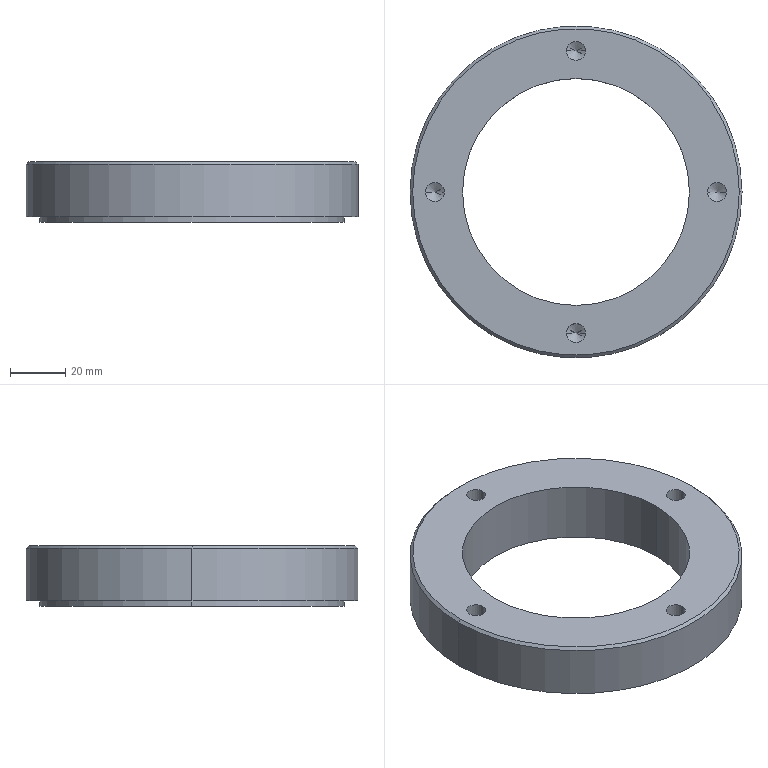Part | SolidWorks | features Chamfer 1, CirPattern 1, FlatPattern 1, HoleWzd 1, ICE 1, SMBaseFlange 1, SheetMetal 1 | 1 solid | 27 faces | box 120 x 120 x 22 mm | volume 125864 mm3 | cylinder 14 | cone 10 | plane 3 | commonest cylinder face diameters 6.8 x8 82 x2 110 x2 120 x2
STEP:
#1=CARTESIAN_POINT('',(-3.4,51.,-19.75));
#2=VERTEX_POINT('',#1);
#3=CARTESIAN_POINT('',(3.4,51.,-19.75));
#4=VERTEX_POINT('',#3);
#5=CARTESIAN_POINT('',(0.,51.,-19.75));
#6=DIRECTION('',(0.,0.,1.));
#7=DIRECTION('',(1.,0.,0.));
#8=AXIS2_PLACEMENT_3D('',#5,#6,#7);
#9=CIRCLE('',#8,3.4);
#10=EDGE_CURVE('',#2,#4,#9,.T.);
#11=ORIENTED_EDGE('',*,*,#10,.F.);
#12=CARTESIAN_POINT('',(-3.4,51.,0.));
#13=VERTEX_POINT('',#12);
#14=CARTESIAN_POINT('',(-3.4,51.,0.));
#15=DIRECTION('',(0.,0.,1.));
#16=VECTOR('',#15,1000.);
#17=LINE('',#14,#16);
#18=EDGE_CURVE('',#2,#13,#17,.T.);
#19=ORIENTED_EDGE('',*,*,#18,.T.);
#20=CARTESIAN_POINT('',(3.4,51.,0.));
#21=VERTEX_POINT('',#20);
#22=CARTESIAN_POINT('',(0.,51.,0.));
#23=DIRECTION('',(0.,0.,1.));
#24=DIRECTION('',(1.,0.,0.));
#25=AXIS2_PLACEMENT_3D('',#22,#23,#24);
#26=CIRCLE('',#25,3.4);
#27=EDGE_CURVE('',#13,#21,#26,.T.);
#28=ORIENTED_EDGE('',*,*,#27,.T.);
#29=CARTESIAN_POINT('',(3.4,51.,0.));
#30=DIRECTION('',(0.,0.,1.));
#31=VECTOR('',#30,1000.);
#32=LINE('',#29,#31);
#33=EDGE_CURVE('',#4,#21,#32,.T.);
#34=ORIENTED_EDGE('',*,*,#33,.F.);
#35=EDGE_LOOP('',(#11,#19,#28,#34));
#36=FACE_OUTER_BOUND('',#35,.T.);
#37=CARTESIAN_POINT('',(0.,51.,0.));
#38=DIRECTION('',(0.,0.,1.));
#39=DIRECTION('',(1.,0.,0.));
#40=AXIS2_PLACEMENT_3D('',#37,#38,#39);
#41=CYLINDRICAL_SURFACE('',#40,3.4);
#42=ADVANCED_FACE('',(#36),#41,.F.);
#43=CARTESIAN_POINT('',(0.,51.,-21.793));
#44=VERTEX_POINT('',#43);
#45=CARTESIAN_POINT('',(3.4,51.,-19.75));
#46=DIRECTION('',(0.8572,0.,0.515));
#47=VECTOR('',#46,1000.);
#48=LINE('',#45,#47);
#49=EDGE_CURVE('',#44,#4,#48,.T.);
#50=ORIENTED_EDGE('',*,*,#49,.F.);
#51=CARTESIAN_POINT('',(-3.4,51.,-19.75));
#52=DIRECTION('',(-0.8572,0.,0.515));
#53=VECTOR('',#52,1000.);
#54=LINE('',#51,#53);
#55=EDGE_CURVE('',#44,#2,#54,.T.);
#56=ORIENTED_EDGE('',*,*,#55,.T.);
#57=ORIENTED_EDGE('',*,*,#10,.T.);
#58=EDGE_LOOP('',(#50,#56,#57));
#59=FACE_OUTER_BOUND('',#58,.T.);
#60=CARTESIAN_POINT('',(0.,51.,-19.75));
#61=DIRECTION('',(0.,0.,1.));
#62=DIRECTION('',(1.,0.,0.));
#63=AXIS2_PLACEMENT_3D('',#60,#61,#62);
#64=CONICAL_SURFACE('',#63,3.4,1.03);
#65=ADVANCED_FACE('',(#59),#64,.F.);
#66=CARTESIAN_POINT('',(-54.4,0.,-19.75));
#67=VERTEX_POINT('',#66);
#68=CARTESIAN_POINT('',(-47.6,0.,-19.75));
#69=VERTEX_POINT('',#68);
#70=CARTESIAN_POINT('',(-51.,0.,-19.75));
#71=DIRECTION('',(0.,0.,1.));
#72=DIRECTION('',(1.,0.,0.));
#73=AXIS2_PLACEMENT_3D('',#70,#71,#72);
#74=CIRCLE('',#73,3.4);
#75=EDGE_CURVE('',#67,#69,#74,.T.);
#76=ORIENTED_EDGE('',*,*,#75,.F.);
#77=CARTESIAN_POINT('',(-54.4,0.,0.));
#78=VERTEX_POINT('',#77);
#79=CARTESIAN_POINT('',(-54.4,0.,0.));
#80=DIRECTION('',(0.,0.,1.));
#81=VECTOR('',#80,1000.);
#82=LINE('',#79,#81);
#83=EDGE_CURVE('',#67,#78,#82,.T.);
#84=ORIENTED_EDGE('',*,*,#83,.T.);
#85=CARTESIAN_POINT('',(-47.6,0.,0.));
#86=VERTEX_POINT('',#85);
#87=CARTESIAN_POINT('',(-51.,0.,0.));
#88=DIRECTION('',(0.,0.,1.));
#89=DIRECTION('',(1.,0.,0.));
#90=AXIS2_PLACEMENT_3D('',#87,#88,#89);
#91=CIRCLE('',#90,3.4);
#92=EDGE_CURVE('',#78,#86,#91,.T.);
#93=ORIENTED_EDGE('',*,*,#92,.T.);
#94=CARTESIAN_POINT('',(-47.6,0.,0.));
#95=DIRECTION('',(0.,0.,1.));
#96=VECTOR('',#95,1000.);
#97=LINE('',#94,#96);
#98=EDGE_CURVE('',#69,#86,#97,.T.);
#99=ORIENTED_EDGE('',*,*,#98,.F.);
#100=EDGE_LOOP('',(#76,#84,#93,#99));
#101=FACE_OUTER_BOUND('',#100,.T.);
#102=CARTESIAN_POINT('',(-51.,0.,0.));
#103=DIRECTION('',(0.,0.,1.));
#104=DIRECTION('',(1.,0.,0.));
#105=AXIS2_PLACEMENT_3D('',#102,#103,#104);
#106=CYLINDRICAL_SURFACE('',#105,3.4);
#107=ADVANCED_FACE('',(#101),#106,.F.);
#108=CARTESIAN_POINT('',(-51.,0.,-21.793));
#109=VERTEX_POINT('',#108);
#110=CARTESIAN_POINT('',(-47.6,0.,-19.75));
#111=DIRECTION('',(0.8572,0.,0.515));
#112=VECTOR('',#111,1000.);
#113=LINE('',#110,#112);
#114=EDGE_CURVE('',#109,#69,#113,.T.);
#115=ORIENTED_EDGE('',*,*,#114,.F.);
#116=CARTESIAN_POINT('',(-54.4,0.,-19.75));
#117=DIRECTION('',(-0.8572,0.,0.515));
#118=VECTOR('',#117,1000.);
#119=LINE('',#116,#118);
#120=EDGE_CURVE('',#109,#67,#119,.T.);
#121=ORIENTED_EDGE('',*,*,#120,.T.);
#122=ORIENTED_EDGE('',*,*,#75,.T.);
#123=EDGE_LOOP('',(#115,#121,#122));
#124=FACE_OUTER_BOUND('',#123,.T.);
#125=CARTESIAN_POINT('',(-51.,0.,-19.75));
#126=DIRECTION('',(0.,0.,1.));
#127=DIRECTION('',(1.,0.,0.));
#128=AXIS2_PLACEMENT_3D('',#125,#126,#127);
#129=CONICAL_SURFACE('',#128,3.4,1.03);
#130=ADVANCED_FACE('',(#124),#129,.F.);
#131=CARTESIAN_POINT('',(-3.4,-51.,-19.75));
#132=VERTEX_POINT('',#131);
#133=CARTESIAN_POINT('',(3.4,-51.,-19.75));
#134=VERTEX_POINT('',#133);
#135=CARTESIAN_POINT('',(0.,-51.,-19.75));
#136=DIRECTION('',(0.,0.,1.));
#137=DIRECTION('',(1.,0.,0.));
#138=AXIS2_PLACEMENT_3D('',#135,#136,#137);
#139=CIRCLE('',#138,3.4);
#140=EDGE_CURVE('',#132,#134,#139,.T.);
#141=ORIENTED_EDGE('',*,*,#140,.F.);
#142=CARTESIAN_POINT('',(-3.4,-51.,0.));
#143=VERTEX_POINT('',#142);
#144=CARTESIAN_POINT('',(-3.4,-51.,0.));
#145=DIRECTION('',(0.,0.,1.));
#146=VECTOR('',#145,1000.);
#147=LINE('',#144,#146);
#148=EDGE_CURVE('',#132,#143,#147,.T.);
#149=ORIENTED_EDGE('',*,*,#148,.T.);
#150=CARTESIAN_POINT('',(3.4,-51.,0.));
#151=VERTEX_POINT('',#150);
#152=CARTESIAN_POINT('',(0.,-51.,0.));
#153=DIRECTION('',(0.,0.,1.));
#154=DIRECTION('',(1.,0.,0.));
#155=AXIS2_PLACEMENT_3D('',#152,#153,#154);
#156=CIRCLE('',#155,3.4);
#157=EDGE_CURVE('',#143,#151,#156,.T.);
#158=ORIENTED_EDGE('',*,*,#157,.T.);
#159=CARTESIAN_POINT('',(3.4,-51.,0.));
#160=DIRECTION('',(0.,0.,1.));
#161=VECTOR('',#160,1000.);
#162=LINE('',#159,#161);
#163=EDGE_CURVE('',#134,#151,#162,.T.);
#164=ORIENTED_EDGE('',*,*,#163,.F.);
#165=EDGE_LOOP('',(#141,#149,#158,#164));
#166=FACE_OUTER_BOUND('',#165,.T.);
#167=CARTESIAN_POINT('',(0.,-51.,0.));
#168=DIRECTION('',(0.,0.,1.));
#169=DIRECTION('',(1.,0.,0.));
#170=AXIS2_PLACEMENT_3D('',#167,#168,#169);
#171=CYLINDRICAL_SURFACE('',#170,3.4);
#172=ADVANCED_FACE('',(#166),#171,.F.);
#173=CARTESIAN_POINT('',(0.,-51.,-21.793));
#174=VERTEX_POINT('',#173);
#175=CARTESIAN_POINT('',(3.4,-51.,-19.75));
#176=DIRECTION('',(0.8572,0.,0.515));
#177=VECTOR('',#176,1000.);
#178=LINE('',#175,#177);
#179=EDGE_CURVE('',#174,#134,#178,.T.);
#180=ORIENTED_EDGE('',*,*,#179,.F.);
#181=CARTESIAN_POINT('',(-3.4,-51.,-19.75));
#182=DIRECTION('',(-0.8572,0.,0.515));
#183=VECTOR('',#182,1000.);
#184=LINE('',#181,#183);
#185=EDGE_CURVE('',#174,#132,#184,.T.);
#186=ORIENTED_EDGE('',*,*,#185,.T.);
#187=ORIENTED_EDGE('',*,*,#140,.T.);
#188=EDGE_LOOP('',(#180,#186,#187));
#189=FACE_OUTER_BOUND('',#188,.T.);
#190=CARTESIAN_POINT('',(0.,-51.,-19.75));
#191=DIRECTION('',(0.,0.,1.));
#192=DIRECTION('',(1.,0.,0.));
#193=AXIS2_PLACEMENT_3D('',#190,#191,#192);
#194=CONICAL_SURFACE('',#193,3.4,1.03);
#195=ADVANCED_FACE('',(#189),#194,.F.);
#196=CARTESIAN_POINT('',(47.6,0.,-19.75));
#197=VERTEX_POINT('',#196);
#198=CARTESIAN_POINT('',(54.4,0.,-19.75));
#199=VERTEX_POINT('',#198);
#200=CARTESIAN_POINT('',(51.,0.,-19.75));
#201=DIRECTION('',(0.,0.,1.));
#202=DIRECTION('',(1.,0.,0.));
#203=AXIS2_PLACEMENT_3D('',#200,#201,#202);
#204=CIRCLE('',#203,3.4);
#205=EDGE_CURVE('',#197,#199,#204,.T.);
#206=ORIENTED_EDGE('',*,*,#205,.F.);
#207=CARTESIAN_POINT('',(47.6,0.,0.));
#208=VERTEX_POINT('',#207);
#209=CARTESIAN_POINT('',(47.6,0.,0.));
#210=DIRECTION('',(0.,0.,1.));
#211=VECTOR('',#210,1000.);
#212=LINE('',#209,#211);
#213=EDGE_CURVE('',#197,#208,#212,.T.);
#214=ORIENTED_EDGE('',*,*,#213,.T.);
#215=CARTESIAN_POINT('',(54.4,0.,0.));
#216=VERTEX_POINT('',#215);
#217=CARTESIAN_POINT('',(51.,0.,0.));
#218=DIRECTION('',(0.,0.,1.));
#219=DIRECTION('',(1.,0.,0.));
#220=AXIS2_PLACEMENT_3D('',#217,#218,#219);
#221=CIRCLE('',#220,3.4);
#222=EDGE_CURVE('',#208,#216,#221,.T.);
#223=ORIENTED_EDGE('',*,*,#222,.T.);
#224=CARTESIAN_POINT('',(54.4,0.,0.));
#225=DIRECTION('',(0.,0.,1.));
#226=VECTOR('',#225,1000.);
#227=LINE('',#224,#226);
#228=EDGE_CURVE('',#199,#216,#227,.T.);
#229=ORIENTED_EDGE('',*,*,#228,.F.);
#230=EDGE_LOOP('',(#206,#214,#223,#229));
#231=FACE_OUTER_BOUND('',#230,.T.);
#232=CARTESIAN_POINT('',(51.,0.,0.));
#233=DIRECTION('',(0.,0.,1.));
#234=DIRECTION('',(1.,0.,0.));
#235=AXIS2_PLACEMENT_3D('',#232,#233,#234);
#236=CYLINDRICAL_SURFACE('',#235,3.4);
#237=ADVANCED_FACE('',(#231),#236,.F.);
#238=CARTESIAN_POINT('',(51.,0.,-21.793));
#239=VERTEX_POINT('',#238);
#240=CARTESIAN_POINT('',(54.4,0.,-19.75));
#241=DIRECTION('',(0.8572,0.,0.515));
#242=VECTOR('',#241,1000.);
#243=LINE('',#240,#242);
#244=EDGE_CURVE('',#239,#199,#243,.T.);
#245=ORIENTED_EDGE('',*,*,#244,.F.);
#246=CARTESIAN_POINT('',(47.6,0.,-19.75));
#247=DIRECTION('',(-0.8572,0.,0.515));
#248=VECTOR('',#247,1000.);
#249=LINE('',#246,#248);
#250=EDGE_CURVE('',#239,#197,#249,.T.);
#251=ORIENTED_EDGE('',*,*,#250,.T.);
#252=ORIENTED_EDGE('',*,*,#205,.T.);
#253=EDGE_LOOP('',(#245,#251,#252));
#254=FACE_OUTER_BOUND('',#253,.T.);
#255=CARTESIAN_POINT('',(51.,0.,-19.75));
#256=DIRECTION('',(0.,0.,1.));
#257=DIRECTION('',(1.,0.,0.));
#258=AXIS2_PLACEMENT_3D('',#255,#256,#257);
#259=CONICAL_SURFACE('',#258,3.4,1.03);
#260=ADVANCED_FACE('',(#254),#259,.F.);
#261=CARTESIAN_POINT('',(59.,0.,0.));
#262=VERTEX_POINT('',#261);
#263=CARTESIAN_POINT('',(-59.,0.,0.));
#264=VERTEX_POINT('',#263);
#265=CARTESIAN_POINT('',(0.,0.,0.));
#266=DIRECTION('',(0.,0.,1.));
#267=DIRECTION('',(1.,0.,0.));
#268=AXIS2_PLACEMENT_3D('',#265,#266,#267);
#269=CIRCLE('',#268,59.);
#270=EDGE_CURVE('',#262,#264,#269,.T.);
#271=ORIENTED_EDGE('',*,*,#270,.F.);
#272=CARTESIAN_POINT('',(60.,0.,-1.));
#273=VERTEX_POINT('',#272);
#274=CARTESIAN_POINT('',(59.,0.,0.));
#275=DIRECTION('',(0.7071,0.,-0.7071));
#276=VECTOR('',#275,1000.);
#277=LINE('',#274,#276);
#278=EDGE_CURVE('',#262,#273,#277,.T.);
#279=ORIENTED_EDGE('',*,*,#278,.T.);
#280=CARTESIAN_POINT('',(-60.,0.,-1.));
#281=VERTEX_POINT('',#280);
#282=CARTESIAN_POINT('',(0.,0.,-1.));
#283=DIRECTION('',(0.,0.,-1.));
#284=DIRECTION('',(1.,0.,0.));
#285=AXIS2_PLACEMENT_3D('',#282,#283,#284);
#286=CIRCLE('',#285,60.);
#287=EDGE_CURVE('',#281,#273,#286,.T.);
#288=ORIENTED_EDGE('',*,*,#287,.F.);
#289=CARTESIAN_POINT('',(-59.,0.,0.));
#290=DIRECTION('',(-0.7071,0.,-0.7071));
#291=VECTOR('',#290,1000.);
#292=LINE('',#289,#291);
#293=EDGE_CURVE('',#264,#281,#292,.T.);
#294=ORIENTED_EDGE('',*,*,#293,.F.);
#295=EDGE_LOOP('',(#271,#279,#288,#294));
#296=FACE_OUTER_BOUND('',#295,.T.);
#297=CARTESIAN_POINT('',(0.,0.,0.));
#298=DIRECTION('',(0.,0.,-1.));
#299=DIRECTION('',(-1.,0.,0.));
#300=AXIS2_PLACEMENT_3D('',#297,#298,#299);
#301=CONICAL_SURFACE('',#300,59.,0.7854);
#302=ADVANCED_FACE('',(#296),#301,.T.);
#303=CARTESIAN_POINT('',(-55.,0.,-22.));
#304=VERTEX_POINT('',#303);
#305=CARTESIAN_POINT('',(55.,0.,-22.));
#306=VERTEX_POINT('',#305);
#307=CARTESIAN_POINT('',(0.,0.,-22.));
#308=DIRECTION('',(0.,0.,-1.));
#309=DIRECTION('',(-1.,0.,0.));
#310=AXIS2_PLACEMENT_3D('',#307,#308,#309);
#311=CIRCLE('',#310,55.);
#312=EDGE_CURVE('',#304,#306,#311,.T.);
#313=ORIENTED_EDGE('',*,*,#312,.F.);
#314=CARTESIAN_POINT('',(-55.,0.,-20.));
#315=VERTEX_POINT('',#314);
#316=CARTESIAN_POINT('',(-55.,0.,-22.));
#317=DIRECTION('',(0.,0.,1.));
#318=VECTOR('',#317,1000.);
#319=LINE('',#316,#318);
#320=EDGE_CURVE('',#304,#315,#319,.T.);
#321=ORIENTED_EDGE('',*,*,#320,.T.);
#322=CARTESIAN_POINT('',(55.,0.,-20.));
#323=VERTEX_POINT('',#322);
#324=CARTESIAN_POINT('',(0.,0.,-20.));
#325=DIRECTION('',(0.,0.,-1.));
#326=DIRECTION('',(-1.,0.,0.));
#327=AXIS2_PLACEMENT_3D('',#324,#325,#326);
#328=CIRCLE('',#327,55.);
#329=EDGE_CURVE('',#315,#323,#328,.T.);
#330=ORIENTED_EDGE('',*,*,#329,.T.);
#331=CARTESIAN_POINT('',(55.,0.,-22.));
#332=DIRECTION('',(0.,0.,1.));
#333=VECTOR('',#332,1000.);
#334=LINE('',#331,#333);
#335=EDGE_CURVE('',#306,#323,#334,.T.);
#336=ORIENTED_EDGE('',*,*,#335,.F.);
#337=EDGE_LOOP('',(#313,#321,#330,#336));
#338=FACE_OUTER_BOUND('',#337,.T.);
#339=CARTESIAN_POINT('',(0.,0.,-22.));
#340=DIRECTION('',(0.,0.,1.));
#341=DIRECTION('',(1.,0.,0.));
#342=AXIS2_PLACEMENT_3D('',#339,#340,#341);
#343=CYLINDRICAL_SURFACE('',#342,55.);
#344=ADVANCED_FACE('',(#338),#343,.T.);
#345=CARTESIAN_POINT('',(41.,0.,-22.));
#346=VERTEX_POINT('',#345);
#347=CARTESIAN_POINT('',(-41.,0.,-22.));
#348=VERTEX_POINT('',#347);
#349=CARTESIAN_POINT('',(0.,0.,-22.));
#350=DIRECTION('',(0.,0.,-1.));
#351=DIRECTION('',(-1.,0.,0.));
#352=AXIS2_PLACEMENT_3D('',#349,#350,#351);
#353=CIRCLE('',#352,41.);
#354=EDGE_CURVE('',#346,#348,#353,.T.);
#355=ORIENTED_EDGE('',*,*,#354,.T.);
#356=CARTESIAN_POINT('',(-41.,0.,0.));
#357=VERTEX_POINT('',#356);
#358=CARTESIAN_POINT('',(-41.,0.,-20.));
#359=DIRECTION('',(0.,0.,1.));
#360=VECTOR('',#359,1000.);
#361=LINE('',#358,#360);
#362=EDGE_CURVE('',#348,#357,#361,.T.);
#363=ORIENTED_EDGE('',*,*,#362,.T.);
#364=CARTESIAN_POINT('',(41.,0.,0.));
#365=VERTEX_POINT('',#364);
#366=CARTESIAN_POINT('',(0.,0.,0.));
#367=DIRECTION('',(0.,0.,1.));
#368=DIRECTION('',(1.,0.,0.));
#369=AXIS2_PLACEMENT_3D('',#366,#367,#368);
#370=CIRCLE('',#369,41.);
#371=EDGE_CURVE('',#357,#365,#370,.T.);
#372=ORIENTED_EDGE('',*,*,#371,.T.);
#373=CARTESIAN_POINT('',(41.,0.,-20.));
#374=DIRECTION('',(0.,0.,1.));
#375=VECTOR('',#374,1000.);
#376=LINE('',#373,#375);
#377=EDGE_CURVE('',#346,#365,#376,.T.);
#378=ORIENTED_EDGE('',*,*,#377,.F.);
#379=EDGE_LOOP('',(#355,#363,#372,#378));
#380=FACE_OUTER_BOUND('',#379,.T.);
#381=CARTESIAN_POINT('',(0.,0.,-20.));
#382=DIRECTION('',(0.,0.,1.));
#383=DIRECTION('',(1.,0.,0.));
#384=AXIS2_PLACEMENT_3D('',#381,#382,#383);
#385=CYLINDRICAL_SURFACE('',#384,41.);
#386=ADVANCED_FACE('',(#380),#385,.F.);
#387=CARTESIAN_POINT('',(60.,0.,-20.));
#388=VERTEX_POINT('',#387);
#389=CARTESIAN_POINT('',(-60.,0.,-20.));
#390=VERTEX_POINT('',#389);
#391=CARTESIAN_POINT('',(0.,0.,-20.));
#392=DIRECTION('',(0.,0.,1.));
#393=DIRECTION('',(1.,0.,0.));
#394=AXIS2_PLACEMENT_3D('',#391,#392,#393);
#395=CIRCLE('',#394,60.);
#396=EDGE_CURVE('',#388,#390,#395,.T.);
#397=ORIENTED_EDGE('',*,*,#396,.T.);
#398=CARTESIAN_POINT('',(-60.,0.,-20.));
#399=DIRECTION('',(0.,0.,1.));
#400=VECTOR('',#399,1000.);
#401=LINE('',#398,#400);
#402=EDGE_CURVE('',#390,#281,#401,.T.);
#403=ORIENTED_EDGE('',*,*,#402,.T.);
#404=ORIENTED_EDGE('',*,*,#287,.T.);
#405=CARTESIAN_POINT('',(60.,0.,-20.));
#406=DIRECTION('',(0.,0.,1.));
#407=VECTOR('',#406,1000.);
#408=LINE('',#405,#407);
#409=EDGE_CURVE('',#388,#273,#408,.T.);
#410=ORIENTED_EDGE('',*,*,#409,.F.);
#411=EDGE_LOOP('',(#397,#403,#404,#410));
#412=FACE_OUTER_BOUND('',#411,.T.);
#413=CARTESIAN_POINT('',(0.,0.,-20.));
#414=DIRECTION('',(0.,0.,1.));
#415=DIRECTION('',(1.,0.,0.));
#416=AXIS2_PLACEMENT_3D('',#413,#414,#415);
#417=CYLINDRICAL_SURFACE('',#416,60.);
#418=ADVANCED_FACE('',(#412),#417,.T.);
#419=ORIENTED_EDGE('',*,*,#402,.F.);
#420=CARTESIAN_POINT('',(0.,0.,-20.));
#421=DIRECTION('',(0.,0.,1.));
#422=DIRECTION('',(1.,0.,0.));
#423=AXIS2_PLACEMENT_3D('',#420,#421,#422);
#424=CIRCLE('',#423,60.);
#425=EDGE_CURVE('',#390,#388,#424,.T.);
#426=ORIENTED_EDGE('',*,*,#425,.T.);
#427=ORIENTED_EDGE('',*,*,#409,.T.);
#428=CARTESIAN_POINT('',(0.,0.,-1.));
#429=DIRECTION('',(0.,0.,-1.));
#430=DIRECTION('',(1.,0.,0.));
#431=AXIS2_PLACEMENT_3D('',#428,#429,#430);
#432=CIRCLE('',#431,60.);
#433=EDGE_CURVE('',#273,#281,#432,.T.);
#434=ORIENTED_EDGE('',*,*,#433,.T.);
#435=EDGE_LOOP('',(#419,#426,#427,#434));
#436=FACE_OUTER_BOUND('',#435,.T.);
#437=CARTESIAN_POINT('',(0.,0.,-20.));
#438=DIRECTION('',(0.,0.,1.));
#439=DIRECTION('',(1.,0.,0.));
#440=AXIS2_PLACEMENT_3D('',#437,#438,#439);
#441=CYLINDRICAL_SURFACE('',#440,60.);
#442=ADVANCED_FACE('',(#436),#441,.T.);
#443=CARTESIAN_POINT('',(0.,0.,-20.));
#444=DIRECTION('',(0.,0.,-1.));
#445=DIRECTION('',(-1.,0.,0.));
#446=AXIS2_PLACEMENT_3D('',#443,#444,#445);
#447=CIRCLE('',#446,55.);
#448=EDGE_CURVE('',#323,#315,#447,.T.);
#449=ORIENTED_EDGE('',*,*,#448,.F.);
#450=ORIENTED_EDGE('',*,*,#329,.F.);
#451=EDGE_LOOP('',(#449,#450));
#452=FACE_BOUND('',#451,.T.);
#453=ORIENTED_EDGE('',*,*,#396,.F.);
#454=ORIENTED_EDGE('',*,*,#425,.F.);
#455=EDGE_LOOP('',(#453,#454));
#456=FACE_OUTER_BOUND('',#455,.T.);
#457=CARTESIAN_POINT('',(0.,0.,-20.));
#458=DIRECTION('',(0.,0.,1.));
#459=DIRECTION('',(1.,0.,0.));
#460=AXIS2_PLACEMENT_3D('',#457,#458,#459);
#461=PLANE('',#460);
#462=ADVANCED_FACE('',(#452,#456),#461,.F.);
#463=CARTESIAN_POINT('',(0.,51.,0.));
#464=DIRECTION('',(0.,0.,1.));
#465=DIRECTION('',(1.,0.,0.));
#466=AXIS2_PLACEMENT_3D('',#463,#464,#465);
#467=CIRCLE('',#466,3.4);
#468=EDGE_CURVE('',#21,#13,#467,.T.);
#469=ORIENTED_EDGE('',*,*,#468,.F.);
#470=ORIENTED_EDGE('',*,*,#27,.F.);
#471=EDGE_LOOP('',(#469,#470));
#472=FACE_BOUND('',#471,.T.);
#473=CARTESIAN_POINT('',(-51.,0.,0.));
#474=DIRECTION('',(0.,0.,1.));
#475=DIRECTION('',(1.,0.,0.));
#476=AXIS2_PLACEMENT_3D('',#473,#474,#475);
#477=CIRCLE('',#476,3.4);
#478=EDGE_CURVE('',#86,#78,#477,.T.);
#479=ORIENTED_EDGE('',*,*,#478,.F.);
#480=ORIENTED_EDGE('',*,*,#92,.F.);
#481=EDGE_LOOP('',(#479,#480));
#482=FACE_BOUND('',#481,.T.);
#483=CARTESIAN_POINT('',(0.,-51.,0.));
#484=DIRECTION('',(0.,0.,1.));
#485=DIRECTION('',(1.,0.,0.));
#486=AXIS2_PLACEMENT_3D('',#483,#484,#485);
#487=CIRCLE('',#486,3.4);
#488=EDGE_CURVE('',#151,#143,#487,.T.);
#489=ORIENTED_EDGE('',*,*,#488,.F.);
#490=ORIENTED_EDGE('',*,*,#157,.F.);
#491=EDGE_LOOP('',(#489,#490));
#492=FACE_BOUND('',#491,.T.);
#493=CARTESIAN_POINT('',(51.,0.,0.));
#494=DIRECTION('',(0.,0.,1.));
#495=DIRECTION('',(1.,0.,0.));
#496=AXIS2_PLACEMENT_3D('',#493,#494,#495);
#497=CIRCLE('',#496,3.4);
#498=EDGE_CURVE('',#216,#208,#497,.T.);
#499=ORIENTED_EDGE('',*,*,#498,.F.);
#500=ORIENTED_EDGE('',*,*,#222,.F.);
#501=EDGE_LOOP('',(#499,#500));
#502=FACE_BOUND('',#501,.T.);
#503=CARTESIAN_POINT('',(0.,0.,0.));
#504=DIRECTION('',(0.,0.,1.));
#505=DIRECTION('',(1.,0.,0.));
#506=AXIS2_PLACEMENT_3D('',#503,#504,#505);
#507=CIRCLE('',#506,59.);
#508=EDGE_CURVE('',#264,#262,#507,.T.);
#509=ORIENTED_EDGE('',*,*,#508,.T.);
#510=ORIENTED_EDGE('',*,*,#270,.T.);
#511=EDGE_LOOP('',(#509,#510));
#512=FACE_OUTER_BOUND('',#511,.T.);
#513=CARTESIAN_POINT('',(0.,0.,0.));
#514=DIRECTION('',(0.,0.,1.));
#515=DIRECTION('',(1.,0.,0.));
#516=AXIS2_PLACEMENT_3D('',#513,#514,#515);
#517=CIRCLE('',#516,41.);
#518=EDGE_CURVE('',#365,#357,#517,.T.);
#519=ORIENTED_EDGE('',*,*,#518,.F.);
#520=ORIENTED_EDGE('',*,*,#371,.F.);
#521=EDGE_LOOP('',(#519,#520));
#522=FACE_BOUND('',#521,.T.);
#523=CARTESIAN_POINT('',(0.,0.,0.));
#524=DIRECTION('',(0.,0.,1.));
#525=DIRECTION('',(1.,0.,0.));
#526=AXIS2_PLACEMENT_3D('',#523,#524,#525);
#527=PLANE('',#526);
#528=ADVANCED_FACE('',(#472,#482,#492,#502,#512,#522),#527,.T.);
#529=ORIENTED_EDGE('',*,*,#362,.F.);
#530=CARTESIAN_POINT('',(0.,0.,-22.));
#531=DIRECTION('',(0.,0.,-1.));
#532=DIRECTION('',(-1.,0.,0.));
#533=AXIS2_PLACEMENT_3D('',#530,#531,#532);
#534=CIRCLE('',#533,41.);
#535=EDGE_CURVE('',#348,#346,#534,.T.);
#536=ORIENTED_EDGE('',*,*,#535,.T.);
#537=ORIENTED_EDGE('',*,*,#377,.T.);
#538=ORIENTED_EDGE('',*,*,#518,.T.);
#539=EDGE_LOOP('',(#529,#536,#537,#538));
#540=FACE_OUTER_BOUND('',#539,.T.);
#541=CARTESIAN_POINT('',(0.,0.,-20.));
#542=DIRECTION('',(0.,0.,1.));
#543=DIRECTION('',(1.,0.,0.));
#544=AXIS2_PLACEMENT_3D('',#541,#542,#543);
#545=CYLINDRICAL_SURFACE('',#544,41.);
#546=ADVANCED_FACE('',(#540),#545,.F.);
#547=CARTESIAN_POINT('',(0.,0.,-22.));
#548=DIRECTION('',(0.,0.,-1.));
#549=DIRECTION('',(-1.,0.,0.));
#550=AXIS2_PLACEMENT_3D('',#547,#548,#549);
#551=CIRCLE('',#550,55.);
#552=EDGE_CURVE('',#306,#304,#551,.T.);
#553=ORIENTED_EDGE('',*,*,#552,.T.);
#554=ORIENTED_EDGE('',*,*,#312,.T.);
#555=EDGE_LOOP('',(#553,#554));
#556=FACE_OUTER_BOUND('',#555,.T.);
#557=ORIENTED_EDGE('',*,*,#354,.F.);
#558=ORIENTED_EDGE('',*,*,#535,.F.);
#559=EDGE_LOOP('',(#557,#558));
#560=FACE_BOUND('',#559,.T.);
#561=CARTESIAN_POINT('',(0.,0.,-22.));
#562=DIRECTION('',(0.,0.,-1.));
#563=DIRECTION('',(-1.,0.,0.));
#564=AXIS2_PLACEMENT_3D('',#561,#562,#563);
#565=PLANE('',#564);
#566=ADVANCED_FACE('',(#556,#560),#565,.T.);
#567=ORIENTED_EDGE('',*,*,#320,.F.);
#568=ORIENTED_EDGE('',*,*,#552,.F.);
#569=ORIENTED_EDGE('',*,*,#335,.T.);
#570=ORIENTED_EDGE('',*,*,#448,.T.);
#571=EDGE_LOOP('',(#567,#568,#569,#570));
#572=FACE_OUTER_BOUND('',#571,.T.);
#573=CARTESIAN_POINT('',(0.,0.,-22.));
#574=DIRECTION('',(0.,0.,1.));
#575=DIRECTION('',(1.,0.,0.));
#576=AXIS2_PLACEMENT_3D('',#573,#574,#575);
#577=CYLINDRICAL_SURFACE('',#576,55.);
#578=ADVANCED_FACE('',(#572),#577,.T.);
#579=ORIENTED_EDGE('',*,*,#278,.F.);
#580=ORIENTED_EDGE('',*,*,#508,.F.);
#581=ORIENTED_EDGE('',*,*,#293,.T.);
#582=ORIENTED_EDGE('',*,*,#433,.F.);
#583=EDGE_LOOP('',(#579,#580,#581,#582));
#584=FACE_OUTER_BOUND('',#583,.T.);
#585=CARTESIAN_POINT('',(0.,0.,0.));
#586=DIRECTION('',(0.,0.,-1.));
#587=DIRECTION('',(-1.,0.,0.));
#588=AXIS2_PLACEMENT_3D('',#585,#586,#587);
#589=CONICAL_SURFACE('',#588,59.,0.7854);
#590=ADVANCED_FACE('',(#584),#589,.T.);
#591=ORIENTED_EDGE('',*,*,#250,.F.);
#592=ORIENTED_EDGE('',*,*,#244,.T.);
#593=CARTESIAN_POINT('',(51.,0.,-19.75));
#594=DIRECTION('',(0.,0.,1.));
#595=DIRECTION('',(1.,0.,0.));
#596=AXIS2_PLACEMENT_3D('',#593,#594,#595);
#597=CIRCLE('',#596,3.4);
#598=EDGE_CURVE('',#199,#197,#597,.T.);
#599=ORIENTED_EDGE('',*,*,#598,.T.);
#600=EDGE_LOOP('',(#591,#592,#599));
#601=FACE_OUTER_BOUND('',#600,.T.);
#602=CARTESIAN_POINT('',(51.,0.,-19.75));
#603=DIRECTION('',(0.,0.,1.));
#604=DIRECTION('',(1.,0.,0.));
#605=AXIS2_PLACEMENT_3D('',#602,#603,#604);
#606=CONICAL_SURFACE('',#605,3.4,1.03);
#607=ADVANCED_FACE('',(#601),#606,.F.);
#608=ORIENTED_EDGE('',*,*,#213,.F.);
#609=ORIENTED_EDGE('',*,*,#598,.F.);
#610=ORIENTED_EDGE('',*,*,#228,.T.);
#611=ORIENTED_EDGE('',*,*,#498,.T.);
#612=EDGE_LOOP('',(#608,#609,#610,#611));
#613=FACE_OUTER_BOUND('',#612,.T.);
#614=CARTESIAN_POINT('',(51.,0.,0.));
#615=DIRECTION('',(0.,0.,1.));
#616=DIRECTION('',(1.,0.,0.));
#617=AXIS2_PLACEMENT_3D('',#614,#615,#616);
#618=CYLINDRICAL_SURFACE('',#617,3.4);
#619=ADVANCED_FACE('',(#613),#618,.F.);
#620=ORIENTED_EDGE('',*,*,#185,.F.);
#621=ORIENTED_EDGE('',*,*,#179,.T.);
#622=CARTESIAN_POINT('',(0.,-51.,-19.75));
#623=DIRECTION('',(0.,0.,1.));
#624=DIRECTION('',(1.,0.,0.));
#625=AXIS2_PLACEMENT_3D('',#622,#623,#624);
#626=CIRCLE('',#625,3.4);
#627=EDGE_CURVE('',#134,#132,#626,.T.);
#628=ORIENTED_EDGE('',*,*,#627,.T.);
#629=EDGE_LOOP('',(#620,#621,#628));
#630=FACE_OUTER_BOUND('',#629,.T.);
#631=CARTESIAN_POINT('',(0.,-51.,-19.75));
#632=DIRECTION('',(0.,0.,1.));
#633=DIRECTION('',(1.,0.,0.));
#634=AXIS2_PLACEMENT_3D('',#631,#632,#633);
#635=CONICAL_SURFACE('',#634,3.4,1.03);
#636=ADVANCED_FACE('',(#630),#635,.F.);
#637=ORIENTED_EDGE('',*,*,#148,.F.);
#638=ORIENTED_EDGE('',*,*,#627,.F.);
#639=ORIENTED_EDGE('',*,*,#163,.T.);
#640=ORIENTED_EDGE('',*,*,#488,.T.);
#641=EDGE_LOOP('',(#637,#638,#639,#640));
#642=FACE_OUTER_BOUND('',#641,.T.);
#643=CARTESIAN_POINT('',(0.,-51.,0.));
#644=DIRECTION('',(0.,0.,1.));
#645=DIRECTION('',(1.,0.,0.));
#646=AXIS2_PLACEMENT_3D('',#643,#644,#645);
#647=CYLINDRICAL_SURFACE('',#646,3.4);
#648=ADVANCED_FACE('',(#642),#647,.F.);
#649=ORIENTED_EDGE('',*,*,#120,.F.);
#650=ORIENTED_EDGE('',*,*,#114,.T.);
#651=CARTESIAN_POINT('',(-51.,0.,-19.75));
#652=DIRECTION('',(0.,0.,1.));
#653=DIRECTION('',(1.,0.,0.));
#654=AXIS2_PLACEMENT_3D('',#651,#652,#653);
#655=CIRCLE('',#654,3.4);
#656=EDGE_CURVE('',#69,#67,#655,.T.);
#657=ORIENTED_EDGE('',*,*,#656,.T.);
#658=EDGE_LOOP('',(#649,#650,#657));
#659=FACE_OUTER_BOUND('',#658,.T.);
#660=CARTESIAN_POINT('',(-51.,0.,-19.75));
#661=DIRECTION('',(0.,0.,1.));
#662=DIRECTION('',(1.,0.,0.));
#663=AXIS2_PLACEMENT_3D('',#660,#661,#662);
#664=CONICAL_SURFACE('',#663,3.4,1.03);
#665=ADVANCED_FACE('',(#659),#664,.F.);
#666=ORIENTED_EDGE('',*,*,#83,.F.);
#667=ORIENTED_EDGE('',*,*,#656,.F.);
#668=ORIENTED_EDGE('',*,*,#98,.T.);
#669=ORIENTED_EDGE('',*,*,#478,.T.);
#670=EDGE_LOOP('',(#666,#667,#668,#669));
#671=FACE_OUTER_BOUND('',#670,.T.);
#672=CARTESIAN_POINT('',(-51.,0.,0.));
#673=DIRECTION('',(0.,0.,1.));
#674=DIRECTION('',(1.,0.,0.));
#675=AXIS2_PLACEMENT_3D('',#672,#673,#674);
#676=CYLINDRICAL_SURFACE('',#675,3.4);
#677=ADVANCED_FACE('',(#671),#676,.F.);
#678=ORIENTED_EDGE('',*,*,#55,.F.);
#679=ORIENTED_EDGE('',*,*,#49,.T.);
#680=CARTESIAN_POINT('',(0.,51.,-19.75));
#681=DIRECTION('',(0.,0.,1.));
#682=DIRECTION('',(1.,0.,0.));
#683=AXIS2_PLACEMENT_3D('',#680,#681,#682);
#684=CIRCLE('',#683,3.4);
#685=EDGE_CURVE('',#4,#2,#684,.T.);
#686=ORIENTED_EDGE('',*,*,#685,.T.);
#687=EDGE_LOOP('',(#678,#679,#686));
#688=FACE_OUTER_BOUND('',#687,.T.);
#689=CARTESIAN_POINT('',(0.,51.,-19.75));
#690=DIRECTION('',(0.,0.,1.));
#691=DIRECTION('',(1.,0.,0.));
#692=AXIS2_PLACEMENT_3D('',#689,#690,#691);
#693=CONICAL_SURFACE('',#692,3.4,1.03);
#694=ADVANCED_FACE('',(#688),#693,.F.);
#695=ORIENTED_EDGE('',*,*,#18,.F.);
#696=ORIENTED_EDGE('',*,*,#685,.F.);
#697=ORIENTED_EDGE('',*,*,#33,.T.);
#698=ORIENTED_EDGE('',*,*,#468,.T.);
#699=EDGE_LOOP('',(#695,#696,#697,#698));
#700=FACE_OUTER_BOUND('',#699,.T.);
#701=CARTESIAN_POINT('',(0.,51.,0.));
#702=DIRECTION('',(0.,0.,1.));
#703=DIRECTION('',(1.,0.,0.));
#704=AXIS2_PLACEMENT_3D('',#701,#702,#703);
#705=CYLINDRICAL_SURFACE('',#704,3.4);
#706=ADVANCED_FACE('',(#700),#705,.F.);
#707=CLOSED_SHELL('',(#42,#65,#107,#130,#172,#195,#237,#260,#302,#344,#386,#418,#442,#462,#528,#546,#566,#578,#590,#607,#619,#636,#648,#665,#677,#694,#706));
#708=MANIFOLD_SOLID_BREP('',#707);
#709=CARTESIAN_POINT('',(0.,0.,0.));
#710=DIRECTION('',(0.,0.,1.));
#711=DIRECTION('',(1.,0.,0.));
#712=AXIS2_PLACEMENT_3D('',#709,#710,#711);
#713=(LENGTH_UNIT()NAMED_UNIT(*)SI_UNIT(.MILLI.,.METRE.));
#714=UNCERTAINTY_MEASURE_WITH_UNIT(LENGTH_MEASURE(0.00001),#713,'','');
#715=(NAMED_UNIT(*)PLANE_ANGLE_UNIT()SI_UNIT($,.RADIAN.));
#716=(NAMED_UNIT(*)SI_UNIT($,.STERADIAN.)SOLID_ANGLE_UNIT());
#717=(GEOMETRIC_REPRESENTATION_CONTEXT(3)GLOBAL_UNCERTAINTY_ASSIGNED_CONTEXT((#714))GLOBAL_UNIT_ASSIGNED_CONTEXT((#713,#715,#716))REPRESENTATION_CONTEXT('',''));
#718=ADVANCED_BREP_SHAPE_REPRESENTATION('',(#708,#712),#717);